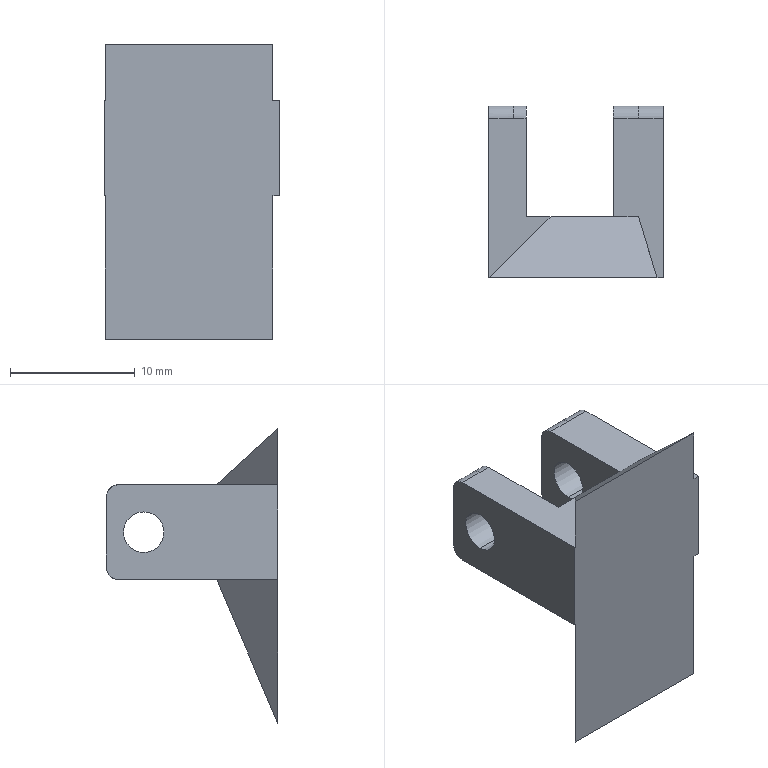Part | SolidWorks | features MirrorStock 1 | 1 solid | 30 faces | box 14 x 13.739 x 23.602 mm | volume 1371 mm3 | plane 18 | cylinder 10 | spline 2 | commonest cylinder face diameters 2 x6 3.25 x4
STEP:
#1=CARTESIAN_POINT('',(-8.5,5.85,-5.425));
#2=VERTEX_POINT('',#1);
#3=CARTESIAN_POINT('',(-8.5,5.85,-2.175));
#4=VERTEX_POINT('',#3);
#5=CARTESIAN_POINT('',(-8.5,5.85,-3.8));
#6=DIRECTION('',(1.,0.,0.));
#7=DIRECTION('',(0.,0.,-1.));
#8=AXIS2_PLACEMENT_3D('',#5,#6,#7);
#9=CIRCLE('',#8,1.625);
#10=EDGE_CURVE('',#2,#4,#9,.T.);
#11=ORIENTED_EDGE('',*,*,#10,.F.);
#12=CARTESIAN_POINT('',(-5.5,5.85,-5.425));
#13=VERTEX_POINT('',#12);
#14=CARTESIAN_POINT('',(-4.1,5.85,-5.425));
#15=DIRECTION('',(1.,0.,0.));
#16=VECTOR('',#15,1000.);
#17=LINE('',#14,#16);
#18=EDGE_CURVE('',#2,#13,#17,.T.);
#19=ORIENTED_EDGE('',*,*,#18,.T.);
#20=CARTESIAN_POINT('',(-5.5,5.85,-2.175));
#21=VERTEX_POINT('',#20);
#22=CARTESIAN_POINT('',(-5.5,5.85,-3.8));
#23=DIRECTION('',(-1.,0.,0.));
#24=DIRECTION('',(0.,0.,-1.));
#25=AXIS2_PLACEMENT_3D('',#22,#23,#24);
#26=CIRCLE('',#25,1.625);
#27=EDGE_CURVE('',#21,#13,#26,.T.);
#28=ORIENTED_EDGE('',*,*,#27,.F.);
#29=CARTESIAN_POINT('',(-4.1,5.85,-2.175));
#30=DIRECTION('',(1.,0.,0.));
#31=VECTOR('',#30,1000.);
#32=LINE('',#29,#31);
#33=EDGE_CURVE('',#4,#21,#32,.T.);
#34=ORIENTED_EDGE('',*,*,#33,.F.);
#35=EDGE_LOOP('',(#11,#19,#28,#34));
#36=FACE_OUTER_BOUND('',#35,.T.);
#37=CARTESIAN_POINT('',(-4.1,5.85,-3.8));
#38=DIRECTION('',(1.,0.,0.));
#39=DIRECTION('',(0.,0.,1.));
#40=AXIS2_PLACEMENT_3D('',#37,#38,#39);
#41=CYLINDRICAL_SURFACE('',#40,1.625);
#42=ADVANCED_FACE('',(#36),#41,.F.);
#43=CARTESIAN_POINT('',(1.5,5.85,-5.425));
#44=VERTEX_POINT('',#43);
#45=CARTESIAN_POINT('',(1.5,5.85,-2.175));
#46=VERTEX_POINT('',#45);
#47=CARTESIAN_POINT('',(1.5,5.85,-3.8));
#48=DIRECTION('',(1.,0.,0.));
#49=DIRECTION('',(0.,1.,0.));
#50=AXIS2_PLACEMENT_3D('',#47,#48,#49);
#51=CIRCLE('',#50,1.625);
#52=EDGE_CURVE('',#44,#46,#51,.T.);
#53=ORIENTED_EDGE('',*,*,#52,.F.);
#54=CARTESIAN_POINT('',(5.5,5.85,-5.425));
#55=VERTEX_POINT('',#54);
#56=CARTESIAN_POINT('',(-4.1,5.85,-5.425));
#57=DIRECTION('',(1.,0.,0.));
#58=VECTOR('',#57,1000.);
#59=LINE('',#56,#58);
#60=EDGE_CURVE('',#44,#55,#59,.T.);
#61=ORIENTED_EDGE('',*,*,#60,.T.);
#62=CARTESIAN_POINT('',(5.5,5.85,-2.175));
#63=VERTEX_POINT('',#62);
#64=CARTESIAN_POINT('',(5.5,5.85,-3.8));
#65=DIRECTION('',(-1.,0.,0.));
#66=DIRECTION('',(0.,0.,1.));
#67=AXIS2_PLACEMENT_3D('',#64,#65,#66);
#68=CIRCLE('',#67,1.625);
#69=EDGE_CURVE('',#63,#55,#68,.T.);
#70=ORIENTED_EDGE('',*,*,#69,.F.);
#71=CARTESIAN_POINT('',(-4.1,5.85,-2.175));
#72=DIRECTION('',(1.,0.,0.));
#73=VECTOR('',#72,1000.);
#74=LINE('',#71,#73);
#75=EDGE_CURVE('',#46,#63,#74,.T.);
#76=ORIENTED_EDGE('',*,*,#75,.F.);
#77=EDGE_LOOP('',(#53,#61,#70,#76));
#78=FACE_OUTER_BOUND('',#77,.T.);
#79=CARTESIAN_POINT('',(-4.1,5.85,-3.8));
#80=DIRECTION('',(1.,0.,0.));
#81=DIRECTION('',(0.,0.,1.));
#82=AXIS2_PLACEMENT_3D('',#79,#80,#81);
#83=CYLINDRICAL_SURFACE('',#82,1.625);
#84=ADVANCED_FACE('',(#78),#83,.F.);
#85=CARTESIAN_POINT('',(-3.5,0.,0.));
#86=VERTEX_POINT('',#85);
#87=CARTESIAN_POINT('',(-8.444,-4.889,4.494));
#88=VERTEX_POINT('',#87);
#89=CARTESIAN_POINT('',(-7.066,-3.527,3.241));
#90=DIRECTION('',(-0.5972,-0.5906,0.5428));
#91=VECTOR('',#90,1000.);
#92=LINE('',#89,#91);
#93=EDGE_CURVE('',#86,#88,#92,.T.);
#94=ORIENTED_EDGE('',*,*,#93,.F.);
#95=CARTESIAN_POINT('',(-8.444,-4.889,0.));
#96=VERTEX_POINT('',#95);
#97=CARTESIAN_POINT('',(-3.5,0.,0.));
#98=DIRECTION('',(-0.711,-0.7032,0.));
#99=VECTOR('',#98,1000.);
#100=LINE('',#97,#99);
#101=EDGE_CURVE('',#86,#96,#100,.T.);
#102=ORIENTED_EDGE('',*,*,#101,.T.);
#103=CARTESIAN_POINT('',(-8.444,-4.889,14.285));
#104=DIRECTION('',(0.,0.,-1.));
#105=VECTOR('',#104,1000.);
#106=LINE('',#103,#105);
#107=EDGE_CURVE('',#88,#96,#106,.T.);
#108=ORIENTED_EDGE('',*,*,#107,.F.);
#109=EDGE_LOOP('',(#94,#102,#108));
#110=FACE_OUTER_BOUND('',#109,.T.);
#111=CARTESIAN_POINT('',(-3.5,0.,14.285));
#112=DIRECTION('',(0.7032,-0.711,0.));
#113=DIRECTION('',(0.711,0.7032,0.));
#114=AXIS2_PLACEMENT_3D('',#111,#112,#113);
#115=PLANE('',#114);
#116=ADVANCED_FACE('',(#110),#115,.F.);
#117=CARTESIAN_POINT('',(3.5,0.,-7.6));
#118=VERTEX_POINT('',#117);
#119=CARTESIAN_POINT('',(4.983,-4.889,-19.108));
#120=VERTEX_POINT('',#119);
#121=CARTESIAN_POINT('',(3.264,0.7776,-5.77));
#122=DIRECTION('',(0.1178,-0.3883,-0.914));
#123=VECTOR('',#122,1000.);
#124=LINE('',#121,#123);
#125=EDGE_CURVE('',#118,#120,#124,.T.);
#126=ORIENTED_EDGE('',*,*,#125,.F.);
#127=CARTESIAN_POINT('',(4.983,-4.889,-7.6));
#128=VERTEX_POINT('',#127);
#129=CARTESIAN_POINT('',(3.5,0.,-7.6));
#130=DIRECTION('',(-0.2903,0.9569,0.));
#131=VECTOR('',#130,1000.);
#132=LINE('',#129,#131);
#133=EDGE_CURVE('',#128,#118,#132,.T.);
#134=ORIENTED_EDGE('',*,*,#133,.F.);
#135=CARTESIAN_POINT('',(4.983,-4.889,14.285));
#136=DIRECTION('',(0.,0.,1.));
#137=VECTOR('',#136,1000.);
#138=LINE('',#135,#137);
#139=EDGE_CURVE('',#120,#128,#138,.T.);
#140=ORIENTED_EDGE('',*,*,#139,.F.);
#141=EDGE_LOOP('',(#126,#134,#140));
#142=FACE_OUTER_BOUND('',#141,.T.);
#143=CARTESIAN_POINT('',(3.5,0.,14.285));
#144=DIRECTION('',(-0.9569,-0.2903,0.));
#145=DIRECTION('',(0.2903,-0.9569,0.));
#146=AXIS2_PLACEMENT_3D('',#143,#144,#145);
#147=PLANE('',#146);
#148=ADVANCED_FACE('',(#142),#147,.F.);
#149=ORIENTED_EDGE('',*,*,#133,.T.);
#150=CARTESIAN_POINT('',(1.5,0.,-7.6));
#151=VERTEX_POINT('',#150);
#152=CARTESIAN_POINT('',(0.,0.,-7.6));
#153=DIRECTION('',(1.,0.,0.));
#154=VECTOR('',#153,1000.);
#155=LINE('',#152,#154);
#156=EDGE_CURVE('',#151,#118,#155,.T.);
#157=ORIENTED_EDGE('',*,*,#156,.F.);
#158=CARTESIAN_POINT('',(1.5,7.85,-7.6));
#159=VERTEX_POINT('',#158);
#160=CARTESIAN_POINT('',(1.5,8.85,-7.6));
#161=DIRECTION('',(0.,-1.,0.));
#162=VECTOR('',#161,1000.);
#163=LINE('',#160,#162);
#164=EDGE_CURVE('',#159,#151,#163,.T.);
#165=ORIENTED_EDGE('',*,*,#164,.F.);
#166=CARTESIAN_POINT('',(3.5,7.85,-7.6));
#167=VERTEX_POINT('',#166);
#168=CARTESIAN_POINT('',(0.,7.85,-7.6));
#169=DIRECTION('',(-1.,0.,0.));
#170=VECTOR('',#169,1000.);
#171=LINE('',#168,#170);
#172=EDGE_CURVE('',#167,#159,#171,.T.);
#173=ORIENTED_EDGE('',*,*,#172,.F.);
#174=CARTESIAN_POINT('',(5.5,7.85,-7.6));
#175=VERTEX_POINT('',#174);
#176=CARTESIAN_POINT('',(5.5,7.85,-7.6));
#177=CARTESIAN_POINT('',(4.833,7.85,-7.6));
#178=CARTESIAN_POINT('',(4.167,7.85,-7.6));
#179=CARTESIAN_POINT('',(3.5,7.85,-7.6));
#180=B_SPLINE_CURVE_WITH_KNOTS('',3,(#176,#177,#178,#179),.UNSPECIFIED.,.F.,.F.,(4,4),(0.,1.),.UNSPECIFIED.);
#181=EDGE_CURVE('',#175,#167,#180,.T.);
#182=ORIENTED_EDGE('',*,*,#181,.F.);
#183=CARTESIAN_POINT('',(5.5,-4.889,-7.6));
#184=VERTEX_POINT('',#183);
#185=CARTESIAN_POINT('',(5.5,-9.889,-7.6));
#186=DIRECTION('',(0.,1.,0.));
#187=VECTOR('',#186,1000.);
#188=LINE('',#185,#187);
#189=EDGE_CURVE('',#184,#175,#188,.T.);
#190=ORIENTED_EDGE('',*,*,#189,.F.);
#191=CARTESIAN_POINT('',(0.,-4.889,-7.6));
#192=DIRECTION('',(1.,0.,0.));
#193=VECTOR('',#192,1000.);
#194=LINE('',#191,#193);
#195=EDGE_CURVE('',#128,#184,#194,.T.);
#196=ORIENTED_EDGE('',*,*,#195,.F.);
#197=EDGE_LOOP('',(#149,#157,#165,#173,#182,#190,#196));
#198=FACE_OUTER_BOUND('',#197,.T.);
#199=CARTESIAN_POINT('',(0.,0.,-7.6));
#200=DIRECTION('',(0.,0.,1.));
#201=DIRECTION('',(-1.,0.,0.));
#202=AXIS2_PLACEMENT_3D('',#199,#200,#201);
#203=PLANE('',#202);
#204=ADVANCED_FACE('',(#198),#203,.F.);
#205=CARTESIAN_POINT('',(4.983,-4.889,0.));
#206=VERTEX_POINT('',#205);
#207=CARTESIAN_POINT('',(5.5,-4.889,0.));
#208=VERTEX_POINT('',#207);
#209=CARTESIAN_POINT('',(0.,-4.889,0.));
#210=DIRECTION('',(1.,0.,0.));
#211=VECTOR('',#210,1000.);
#212=LINE('',#209,#211);
#213=EDGE_CURVE('',#206,#208,#212,.T.);
#214=ORIENTED_EDGE('',*,*,#213,.T.);
#215=CARTESIAN_POINT('',(5.5,7.85,0.));
#216=VERTEX_POINT('',#215);
#217=CARTESIAN_POINT('',(5.5,-9.889,0.));
#218=DIRECTION('',(0.,1.,0.));
#219=VECTOR('',#218,1000.);
#220=LINE('',#217,#219);
#221=EDGE_CURVE('',#208,#216,#220,.T.);
#222=ORIENTED_EDGE('',*,*,#221,.T.);
#223=CARTESIAN_POINT('',(3.5,7.85,0.));
#224=VERTEX_POINT('',#223);
#225=CARTESIAN_POINT('',(0.,7.85,0.));
#226=DIRECTION('',(1.,0.,0.));
#227=VECTOR('',#226,1000.);
#228=LINE('',#225,#227);
#229=EDGE_CURVE('',#224,#216,#228,.T.);
#230=ORIENTED_EDGE('',*,*,#229,.F.);
#231=CARTESIAN_POINT('',(1.5,7.85,0.));
#232=VERTEX_POINT('',#231);
#233=CARTESIAN_POINT('',(0.,7.85,0.));
#234=DIRECTION('',(1.,0.,0.));
#235=VECTOR('',#234,1000.);
#236=LINE('',#233,#235);
#237=EDGE_CURVE('',#232,#224,#236,.T.);
#238=ORIENTED_EDGE('',*,*,#237,.F.);
#239=CARTESIAN_POINT('',(1.5,0.,0.));
#240=VERTEX_POINT('',#239);
#241=CARTESIAN_POINT('',(1.5,8.85,0.));
#242=DIRECTION('',(0.,-1.,0.));
#243=VECTOR('',#242,1000.);
#244=LINE('',#241,#243);
#245=EDGE_CURVE('',#232,#240,#244,.T.);
#246=ORIENTED_EDGE('',*,*,#245,.T.);
#247=CARTESIAN_POINT('',(3.5,0.,0.));
#248=VERTEX_POINT('',#247);
#249=CARTESIAN_POINT('',(3.5,0.,0.));
#250=DIRECTION('',(-1.,0.,0.));
#251=VECTOR('',#250,1000.);
#252=LINE('',#249,#251);
#253=EDGE_CURVE('',#248,#240,#252,.T.);
#254=ORIENTED_EDGE('',*,*,#253,.F.);
#255=CARTESIAN_POINT('',(3.5,0.,0.));
#256=DIRECTION('',(0.2903,-0.9569,0.));
#257=VECTOR('',#256,1000.);
#258=LINE('',#255,#257);
#259=EDGE_CURVE('',#248,#206,#258,.T.);
#260=ORIENTED_EDGE('',*,*,#259,.T.);
#261=EDGE_LOOP('',(#214,#222,#230,#238,#246,#254,#260));
#262=FACE_OUTER_BOUND('',#261,.T.);
#263=CARTESIAN_POINT('',(0.,0.,0.));
#264=DIRECTION('',(0.,0.,1.));
#265=DIRECTION('',(-1.,0.,0.));
#266=AXIS2_PLACEMENT_3D('',#263,#264,#265);
#267=PLANE('',#266);
#268=ADVANCED_FACE('',(#262),#267,.T.);
#269=ORIENTED_EDGE('',*,*,#229,.T.);
#270=CARTESIAN_POINT('',(5.5,8.85,-1.));
#271=VERTEX_POINT('',#270);
#272=CARTESIAN_POINT('',(5.5,7.85,-1.));
#273=DIRECTION('',(-1.,0.,0.));
#274=DIRECTION('',(0.,0.,1.));
#275=AXIS2_PLACEMENT_3D('',#272,#273,#274);
#276=CIRCLE('',#275,1.);
#277=EDGE_CURVE('',#216,#271,#276,.T.);
#278=ORIENTED_EDGE('',*,*,#277,.T.);
#279=CARTESIAN_POINT('',(3.5,8.85,-1.));
#280=VERTEX_POINT('',#279);
#281=CARTESIAN_POINT('',(0.,8.85,-1.));
#282=DIRECTION('',(-1.,0.,0.));
#283=VECTOR('',#282,1000.);
#284=LINE('',#281,#283);
#285=EDGE_CURVE('',#271,#280,#284,.T.);
#286=ORIENTED_EDGE('',*,*,#285,.T.);
#287=CARTESIAN_POINT('',(3.5,7.85,-1.));
#288=DIRECTION('',(-1.,0.,0.));
#289=DIRECTION('',(0.,0.,-1.));
#290=AXIS2_PLACEMENT_3D('',#287,#288,#289);
#291=CIRCLE('',#290,1.);
#292=EDGE_CURVE('',#224,#280,#291,.T.);
#293=ORIENTED_EDGE('',*,*,#292,.F.);
#294=EDGE_LOOP('',(#269,#278,#286,#293));
#295=FACE_OUTER_BOUND('',#294,.T.);
#296=CARTESIAN_POINT('',(0.,7.85,-1.));
#297=DIRECTION('',(-1.,0.,0.));
#298=DIRECTION('',(0.,0.,-1.));
#299=AXIS2_PLACEMENT_3D('',#296,#297,#298);
#300=CYLINDRICAL_SURFACE('',#299,1.);
#301=ADVANCED_FACE('',(#295),#300,.T.);
#302=CARTESIAN_POINT('',(-8.5,7.85,0.));
#303=VERTEX_POINT('',#302);
#304=CARTESIAN_POINT('',(-6.5,7.85,0.));
#305=VERTEX_POINT('',#304);
#306=CARTESIAN_POINT('',(-8.5,7.85,0.));
#307=CARTESIAN_POINT('',(-7.833,7.85,0.));
#308=CARTESIAN_POINT('',(-7.167,7.85,0.));
#309=CARTESIAN_POINT('',(-6.5,7.85,0.));
#310=B_SPLINE_CURVE_WITH_KNOTS('',3,(#306,#307,#308,#309),.UNSPECIFIED.,.F.,.F.,(4,4),(0.,1.),.UNSPECIFIED.);
#311=EDGE_CURVE('',#303,#305,#310,.T.);
#312=ORIENTED_EDGE('',*,*,#311,.T.);
#313=CARTESIAN_POINT('',(-6.5,8.85,-1.));
#314=VERTEX_POINT('',#313);
#315=CARTESIAN_POINT('',(-6.5,8.85,-1.));
#316=CARTESIAN_POINT('',(-6.5,8.85,-0.7382));
#317=CARTESIAN_POINT('',(-6.5,8.742,-0.478));
#318=CARTESIAN_POINT('',(-6.5,8.372,-0.1078));
#319=CARTESIAN_POINT('',(-6.5,8.112,0.));
#320=CARTESIAN_POINT('',(-6.5,7.85,0.));
#321=B_SPLINE_CURVE_WITH_KNOTS('',3,(#315,#316,#317,#318,#319,#320),.UNSPECIFIED.,.F.,.F.,(4,2,4),(0.,0.5,1.),.UNSPECIFIED.);
#322=EDGE_CURVE('',#314,#305,#321,.T.);
#323=ORIENTED_EDGE('',*,*,#322,.F.);
#324=CARTESIAN_POINT('',(-8.5,8.85,-1.));
#325=VERTEX_POINT('',#324);
#326=CARTESIAN_POINT('',(-6.5,8.85,-1.));
#327=CARTESIAN_POINT('',(-7.167,8.85,-1.));
#328=CARTESIAN_POINT('',(-7.833,8.85,-1.));
#329=CARTESIAN_POINT('',(-8.5,8.85,-1.));
#330=B_SPLINE_CURVE_WITH_KNOTS('',3,(#326,#327,#328,#329),.UNSPECIFIED.,.F.,.F.,(4,4),(0.,1.),.UNSPECIFIED.);
#331=EDGE_CURVE('',#314,#325,#330,.T.);
#332=ORIENTED_EDGE('',*,*,#331,.T.);
#333=CARTESIAN_POINT('',(-8.5,8.85,-1.));
#334=CARTESIAN_POINT('',(-8.5,8.85,0.));
#335=CARTESIAN_POINT('',(-8.5,7.85,0.));
#336=(BOUNDED_CURVE()B_SPLINE_CURVE(2,(#333,#334,#335),.UNSPECIFIED.,.F.,.F.)B_SPLINE_CURVE_WITH_KNOTS((3,3),(0.,1.),.UNSPECIFIED.)CURVE()GEOMETRIC_REPRESENTATION_ITEM()RATIONAL_B_SPLINE_CURVE((1.,0.7071,1.))REPRESENTATION_ITEM(''));
#337=EDGE_CURVE('',#325,#303,#336,.T.);
#338=ORIENTED_EDGE('',*,*,#337,.T.);
#339=EDGE_LOOP('',(#312,#323,#332,#338));
#340=FACE_OUTER_BOUND('',#339,.T.);
#341=CARTESIAN_POINT('',(-6.3,8.85,-1.));
#342=CARTESIAN_POINT('',(-6.367,8.85,-1.));
#343=CARTESIAN_POINT('',(-6.433,8.85,-1.));
#344=CARTESIAN_POINT('',(-7.167,8.85,-1.));
#345=CARTESIAN_POINT('',(-7.833,8.85,-1.));
#346=CARTESIAN_POINT('',(-8.567,8.85,-1.));
#347=CARTESIAN_POINT('',(-8.633,8.85,-1.));
#348=CARTESIAN_POINT('',(-8.7,8.85,-1.));
#349=CARTESIAN_POINT('',(-6.3,8.85,0.));
#350=CARTESIAN_POINT('',(-6.367,8.85,0.));
#351=CARTESIAN_POINT('',(-6.433,8.85,0.));
#352=CARTESIAN_POINT('',(-7.167,8.85,0.));
#353=CARTESIAN_POINT('',(-7.833,8.85,0.));
#354=CARTESIAN_POINT('',(-8.567,8.85,0.));
#355=CARTESIAN_POINT('',(-8.633,8.85,0.));
#356=CARTESIAN_POINT('',(-8.7,8.85,0.));
#357=CARTESIAN_POINT('',(-6.3,7.85,0.));
#358=CARTESIAN_POINT('',(-6.367,7.85,0.));
#359=CARTESIAN_POINT('',(-6.433,7.85,0.));
#360=CARTESIAN_POINT('',(-7.167,7.85,0.));
#361=CARTESIAN_POINT('',(-7.833,7.85,0.));
#362=CARTESIAN_POINT('',(-8.567,7.85,0.));
#363=CARTESIAN_POINT('',(-8.633,7.85,0.));
#364=CARTESIAN_POINT('',(-8.7,7.85,0.));
#365=(BOUNDED_SURFACE()B_SPLINE_SURFACE(2,3,((#341,#342,#343,#344,#345,#346,#347,#348),(#349,#350,#351,#352,#353,#354,#355,#356),(#357,#358,#359,#360,#361,#362,#363,#364)),.UNSPECIFIED.,.F.,.F.,.F.)B_SPLINE_SURFACE_WITH_KNOTS((3,3),(4,2,2,4),(0.,1.),(-0.1,0.,1.,1.1),.UNSPECIFIED.)GEOMETRIC_REPRESENTATION_ITEM()RATIONAL_B_SPLINE_SURFACE(((1.,1.,1.,1.,1.,1.,1.,1.),(0.7071,0.7071,0.7071,0.7071,0.7071,0.7071,0.7071,0.7071),(1.,1.,1.,1.,1.,1.,1.,1.)))REPRESENTATION_ITEM('')SURFACE());
#366=ADVANCED_FACE('',(#340),#365,.F.);
#367=CARTESIAN_POINT('',(-6.5,7.85,-7.6));
#368=VERTEX_POINT('',#367);
#369=CARTESIAN_POINT('',(-8.5,7.85,-7.6));
#370=VERTEX_POINT('',#369);
#371=CARTESIAN_POINT('',(0.,7.85,-7.6));
#372=DIRECTION('',(-1.,0.,0.));
#373=VECTOR('',#372,1000.);
#374=LINE('',#371,#373);
#375=EDGE_CURVE('',#368,#370,#374,.T.);
#376=ORIENTED_EDGE('',*,*,#375,.T.);
#377=CARTESIAN_POINT('',(-8.5,8.85,-6.6));
#378=VERTEX_POINT('',#377);
#379=CARTESIAN_POINT('',(-8.5,7.85,-6.6));
#380=DIRECTION('',(1.,0.,0.));
#381=DIRECTION('',(0.,0.,-1.));
#382=AXIS2_PLACEMENT_3D('',#379,#380,#381);
#383=CIRCLE('',#382,1.);
#384=EDGE_CURVE('',#370,#378,#383,.T.);
#385=ORIENTED_EDGE('',*,*,#384,.T.);
#386=CARTESIAN_POINT('',(-6.5,8.85,-6.6));
#387=VERTEX_POINT('',#386);
#388=CARTESIAN_POINT('',(-3.5,8.85,-6.6));
#389=DIRECTION('',(1.,0.,0.));
#390=VECTOR('',#389,1000.);
#391=LINE('',#388,#390);
#392=EDGE_CURVE('',#378,#387,#391,.T.);
#393=ORIENTED_EDGE('',*,*,#392,.T.);
#394=CARTESIAN_POINT('',(-6.5,7.85,-6.6));
#395=DIRECTION('',(1.,0.,0.));
#396=DIRECTION('',(0.,-1.,0.));
#397=AXIS2_PLACEMENT_3D('',#394,#395,#396);
#398=CIRCLE('',#397,1.);
#399=EDGE_CURVE('',#368,#387,#398,.T.);
#400=ORIENTED_EDGE('',*,*,#399,.F.);
#401=EDGE_LOOP('',(#376,#385,#393,#400));
#402=FACE_OUTER_BOUND('',#401,.T.);
#403=CARTESIAN_POINT('',(0.,7.85,-6.6));
#404=DIRECTION('',(-1.,0.,0.));
#405=DIRECTION('',(0.,0.,-1.));
#406=AXIS2_PLACEMENT_3D('',#403,#404,#405);
#407=CYLINDRICAL_SURFACE('',#406,1.);
#408=ADVANCED_FACE('',(#402),#407,.T.);
#409=ORIENTED_EDGE('',*,*,#181,.T.);
#410=CARTESIAN_POINT('',(3.5,8.85,-6.6));
#411=VERTEX_POINT('',#410);
#412=CARTESIAN_POINT('',(3.5,8.85,-6.6));
#413=CARTESIAN_POINT('',(3.5,8.85,-6.862));
#414=CARTESIAN_POINT('',(3.5,8.742,-7.122));
#415=CARTESIAN_POINT('',(3.5,8.372,-7.492));
#416=CARTESIAN_POINT('',(3.5,8.112,-7.6));
#417=CARTESIAN_POINT('',(3.5,7.85,-7.6));
#418=B_SPLINE_CURVE_WITH_KNOTS('',3,(#412,#413,#414,#415,#416,#417),.UNSPECIFIED.,.F.,.F.,(4,2,4),(0.,0.5,1.),.UNSPECIFIED.);
#419=EDGE_CURVE('',#411,#167,#418,.T.);
#420=ORIENTED_EDGE('',*,*,#419,.F.);
#421=CARTESIAN_POINT('',(5.5,8.85,-6.6));
#422=VERTEX_POINT('',#421);
#423=CARTESIAN_POINT('',(3.5,8.85,-6.6));
#424=CARTESIAN_POINT('',(4.167,8.85,-6.6));
#425=CARTESIAN_POINT('',(4.833,8.85,-6.6));
#426=CARTESIAN_POINT('',(5.5,8.85,-6.6));
#427=B_SPLINE_CURVE_WITH_KNOTS('',3,(#423,#424,#425,#426),.UNSPECIFIED.,.F.,.F.,(4,4),(0.,1.),.UNSPECIFIED.);
#428=EDGE_CURVE('',#411,#422,#427,.T.);
#429=ORIENTED_EDGE('',*,*,#428,.T.);
#430=CARTESIAN_POINT('',(5.5,8.85,-6.6));
#431=CARTESIAN_POINT('',(5.5,8.85,-7.6));
#432=CARTESIAN_POINT('',(5.5,7.85,-7.6));
#433=(BOUNDED_CURVE()B_SPLINE_CURVE(2,(#430,#431,#432),.UNSPECIFIED.,.F.,.F.)B_SPLINE_CURVE_WITH_KNOTS((3,3),(0.,1.),.UNSPECIFIED.)CURVE()GEOMETRIC_REPRESENTATION_ITEM()RATIONAL_B_SPLINE_CURVE((1.,0.7071,1.))REPRESENTATION_ITEM(''));
#434=EDGE_CURVE('',#422,#175,#433,.T.);
#435=ORIENTED_EDGE('',*,*,#434,.T.);
#436=EDGE_LOOP('',(#409,#420,#429,#435));
#437=FACE_OUTER_BOUND('',#436,.T.);
#438=CARTESIAN_POINT('',(3.3,8.85,-6.6));
#439=CARTESIAN_POINT('',(3.367,8.85,-6.6));
#440=CARTESIAN_POINT('',(3.433,8.85,-6.6));
#441=CARTESIAN_POINT('',(4.167,8.85,-6.6));
#442=CARTESIAN_POINT('',(4.833,8.85,-6.6));
#443=CARTESIAN_POINT('',(5.567,8.85,-6.6));
#444=CARTESIAN_POINT('',(5.633,8.85,-6.6));
#445=CARTESIAN_POINT('',(5.7,8.85,-6.6));
#446=CARTESIAN_POINT('',(3.3,8.85,-7.6));
#447=CARTESIAN_POINT('',(3.367,8.85,-7.6));
#448=CARTESIAN_POINT('',(3.433,8.85,-7.6));
#449=CARTESIAN_POINT('',(4.167,8.85,-7.6));
#450=CARTESIAN_POINT('',(4.833,8.85,-7.6));
#451=CARTESIAN_POINT('',(5.567,8.85,-7.6));
#452=CARTESIAN_POINT('',(5.633,8.85,-7.6));
#453=CARTESIAN_POINT('',(5.7,8.85,-7.6));
#454=CARTESIAN_POINT('',(3.3,7.85,-7.6));
#455=CARTESIAN_POINT('',(3.367,7.85,-7.6));
#456=CARTESIAN_POINT('',(3.433,7.85,-7.6));
#457=CARTESIAN_POINT('',(4.167,7.85,-7.6));
#458=CARTESIAN_POINT('',(4.833,7.85,-7.6));
#459=CARTESIAN_POINT('',(5.567,7.85,-7.6));
#460=CARTESIAN_POINT('',(5.633,7.85,-7.6));
#461=CARTESIAN_POINT('',(5.7,7.85,-7.6));
#462=(BOUNDED_SURFACE()B_SPLINE_SURFACE(2,3,((#438,#439,#440,#441,#442,#443,#444,#445),(#446,#447,#448,#449,#450,#451,#452,#453),(#454,#455,#456,#457,#458,#459,#460,#461)),.UNSPECIFIED.,.F.,.F.,.F.)B_SPLINE_SURFACE_WITH_KNOTS((3,3),(4,2,2,4),(0.,1.),(-0.1,0.,1.,1.1),.UNSPECIFIED.)GEOMETRIC_REPRESENTATION_ITEM()RATIONAL_B_SPLINE_SURFACE(((1.,1.,1.,1.,1.,1.,1.,1.),(0.7071,0.7071,0.7071,0.7071,0.7071,0.7071,0.7071,0.7071),(1.,1.,1.,1.,1.,1.,1.,1.)))REPRESENTATION_ITEM('')SURFACE());
#463=ADVANCED_FACE('',(#437),#462,.F.);
#464=CARTESIAN_POINT('',(-5.5,7.85,0.));
#465=VERTEX_POINT('',#464);
#466=CARTESIAN_POINT('',(-5.5,8.85,-1.));
#467=VERTEX_POINT('',#466);
#468=CARTESIAN_POINT('',(-5.5,7.85,-1.));
#469=DIRECTION('',(-1.,0.,0.));
#470=DIRECTION('',(0.,0.,-1.));
#471=AXIS2_PLACEMENT_3D('',#468,#469,#470);
#472=CIRCLE('',#471,1.);
#473=EDGE_CURVE('',#465,#467,#472,.T.);
#474=ORIENTED_EDGE('',*,*,#473,.T.);
#475=CARTESIAN_POINT('',(0.,8.85,-1.));
#476=DIRECTION('',(-1.,0.,0.));
#477=VECTOR('',#476,1000.);
#478=LINE('',#475,#477);
#479=EDGE_CURVE('',#467,#314,#478,.T.);
#480=ORIENTED_EDGE('',*,*,#479,.T.);
#481=ORIENTED_EDGE('',*,*,#322,.T.);
#482=CARTESIAN_POINT('',(0.,7.85,0.));
#483=DIRECTION('',(1.,0.,0.));
#484=VECTOR('',#483,1000.);
#485=LINE('',#482,#484);
#486=EDGE_CURVE('',#305,#465,#485,.T.);
#487=ORIENTED_EDGE('',*,*,#486,.T.);
#488=EDGE_LOOP('',(#474,#480,#481,#487));
#489=FACE_OUTER_BOUND('',#488,.T.);
#490=CARTESIAN_POINT('',(0.,7.85,-1.));
#491=DIRECTION('',(-1.,0.,0.));
#492=DIRECTION('',(0.,0.,-1.));
#493=AXIS2_PLACEMENT_3D('',#490,#491,#492);
#494=CYLINDRICAL_SURFACE('',#493,1.);
#495=ADVANCED_FACE('',(#489),#494,.T.);
#496=CARTESIAN_POINT('',(-5.5,8.85,-6.6));
#497=VERTEX_POINT('',#496);
#498=CARTESIAN_POINT('',(-5.5,7.85,-7.6));
#499=VERTEX_POINT('',#498);
#500=CARTESIAN_POINT('',(-5.5,7.85,-6.6));
#501=DIRECTION('',(-1.,0.,0.));
#502=DIRECTION('',(0.,0.,-1.));
#503=AXIS2_PLACEMENT_3D('',#500,#501,#502);
#504=CIRCLE('',#503,1.);
#505=EDGE_CURVE('',#497,#499,#504,.T.);
#506=ORIENTED_EDGE('',*,*,#505,.T.);
#507=CARTESIAN_POINT('',(0.,7.85,-7.6));
#508=DIRECTION('',(-1.,0.,0.));
#509=VECTOR('',#508,1000.);
#510=LINE('',#507,#509);
#511=EDGE_CURVE('',#499,#368,#510,.T.);
#512=ORIENTED_EDGE('',*,*,#511,.T.);
#513=ORIENTED_EDGE('',*,*,#399,.T.);
#514=CARTESIAN_POINT('',(-3.5,8.85,-6.6));
#515=DIRECTION('',(1.,0.,0.));
#516=VECTOR('',#515,1000.);
#517=LINE('',#514,#516);
#518=EDGE_CURVE('',#387,#497,#517,.T.);
#519=ORIENTED_EDGE('',*,*,#518,.T.);
#520=EDGE_LOOP('',(#506,#512,#513,#519));
#521=FACE_OUTER_BOUND('',#520,.T.);
#522=CARTESIAN_POINT('',(0.,7.85,-6.6));
#523=DIRECTION('',(-1.,0.,0.));
#524=DIRECTION('',(0.,0.,-1.));
#525=AXIS2_PLACEMENT_3D('',#522,#523,#524);
#526=CYLINDRICAL_SURFACE('',#525,1.);
#527=ADVANCED_FACE('',(#521),#526,.T.);
#528=CARTESIAN_POINT('',(-8.444,-4.889,-7.6));
#529=VERTEX_POINT('',#528);
#530=CARTESIAN_POINT('',(-3.5,0.,-7.6));
#531=VERTEX_POINT('',#530);
#532=CARTESIAN_POINT('',(-3.5,0.,-7.6));
#533=DIRECTION('',(0.711,0.7032,0.));
#534=VECTOR('',#533,1000.);
#535=LINE('',#532,#534);
#536=EDGE_CURVE('',#529,#531,#535,.T.);
#537=ORIENTED_EDGE('',*,*,#536,.T.);
#538=CARTESIAN_POINT('',(-8.444,-4.889,-19.108));
#539=VERTEX_POINT('',#538);
#540=CARTESIAN_POINT('',(-4.852,-1.337,-10.747));
#541=DIRECTION('',(0.3677,0.3636,0.8559));
#542=VECTOR('',#541,1000.);
#543=LINE('',#540,#542);
#544=EDGE_CURVE('',#539,#531,#543,.T.);
#545=ORIENTED_EDGE('',*,*,#544,.F.);
#546=CARTESIAN_POINT('',(-8.444,-4.889,14.285));
#547=DIRECTION('',(0.,0.,-1.));
#548=VECTOR('',#547,1000.);
#549=LINE('',#546,#548);
#550=EDGE_CURVE('',#529,#539,#549,.T.);
#551=ORIENTED_EDGE('',*,*,#550,.F.);
#552=EDGE_LOOP('',(#537,#545,#551));
#553=FACE_OUTER_BOUND('',#552,.T.);
#554=CARTESIAN_POINT('',(-3.5,0.,14.285));
#555=DIRECTION('',(0.7032,-0.711,0.));
#556=DIRECTION('',(0.711,0.7032,0.));
#557=AXIS2_PLACEMENT_3D('',#554,#555,#556);
#558=PLANE('',#557);
#559=ADVANCED_FACE('',(#553),#558,.F.);
#560=ORIENTED_EDGE('',*,*,#172,.T.);
#561=CARTESIAN_POINT('',(1.5,8.85,-6.6));
#562=VERTEX_POINT('',#561);
#563=CARTESIAN_POINT('',(1.5,7.85,-6.6));
#564=DIRECTION('',(1.,0.,0.));
#565=DIRECTION('',(0.,1.,0.));
#566=AXIS2_PLACEMENT_3D('',#563,#564,#565);
#567=CIRCLE('',#566,1.);
#568=EDGE_CURVE('',#159,#562,#567,.T.);
#569=ORIENTED_EDGE('',*,*,#568,.T.);
#570=CARTESIAN_POINT('',(-3.5,8.85,-6.6));
#571=DIRECTION('',(1.,0.,0.));
#572=VECTOR('',#571,1000.);
#573=LINE('',#570,#572);
#574=EDGE_CURVE('',#562,#411,#573,.T.);
#575=ORIENTED_EDGE('',*,*,#574,.T.);
#576=ORIENTED_EDGE('',*,*,#419,.T.);
#577=EDGE_LOOP('',(#560,#569,#575,#576));
#578=FACE_OUTER_BOUND('',#577,.T.);
#579=CARTESIAN_POINT('',(0.,7.85,-6.6));
#580=DIRECTION('',(-1.,0.,0.));
#581=DIRECTION('',(0.,0.,-1.));
#582=AXIS2_PLACEMENT_3D('',#579,#580,#581);
#583=CYLINDRICAL_SURFACE('',#582,1.);
#584=ADVANCED_FACE('',(#578),#583,.T.);
#585=ORIENTED_EDGE('',*,*,#237,.T.);
#586=ORIENTED_EDGE('',*,*,#292,.T.);
#587=CARTESIAN_POINT('',(1.5,8.85,-1.));
#588=VERTEX_POINT('',#587);
#589=CARTESIAN_POINT('',(0.,8.85,-1.));
#590=DIRECTION('',(-1.,0.,0.));
#591=VECTOR('',#590,1000.);
#592=LINE('',#589,#591);
#593=EDGE_CURVE('',#280,#588,#592,.T.);
#594=ORIENTED_EDGE('',*,*,#593,.T.);
#595=CARTESIAN_POINT('',(1.5,7.85,-1.));
#596=DIRECTION('',(1.,0.,0.));
#597=DIRECTION('',(0.,1.,0.));
#598=AXIS2_PLACEMENT_3D('',#595,#596,#597);
#599=CIRCLE('',#598,1.);
#600=EDGE_CURVE('',#588,#232,#599,.T.);
#601=ORIENTED_EDGE('',*,*,#600,.T.);
#602=EDGE_LOOP('',(#585,#586,#594,#601));
#603=FACE_OUTER_BOUND('',#602,.T.);
#604=CARTESIAN_POINT('',(0.,7.85,-1.));
#605=DIRECTION('',(-1.,0.,0.));
#606=DIRECTION('',(0.,0.,-1.));
#607=AXIS2_PLACEMENT_3D('',#604,#605,#606);
#608=CYLINDRICAL_SURFACE('',#607,1.);
#609=ADVANCED_FACE('',(#603),#608,.T.);
#610=CARTESIAN_POINT('',(5.5,8.85,0.));
#611=DIRECTION('',(0.,0.,1.));
#612=VECTOR('',#611,1000.);
#613=LINE('',#610,#612);
#614=EDGE_CURVE('',#422,#271,#613,.T.);
#615=ORIENTED_EDGE('',*,*,#614,.F.);
#616=ORIENTED_EDGE('',*,*,#428,.F.);
#617=ORIENTED_EDGE('',*,*,#574,.F.);
#618=CARTESIAN_POINT('',(1.5,8.85,-7.6));
#619=DIRECTION('',(0.,0.,1.));
#620=VECTOR('',#619,1000.);
#621=LINE('',#618,#620);
#622=EDGE_CURVE('',#562,#588,#621,.T.);
#623=ORIENTED_EDGE('',*,*,#622,.T.);
#624=ORIENTED_EDGE('',*,*,#593,.F.);
#625=ORIENTED_EDGE('',*,*,#285,.F.);
#626=EDGE_LOOP('',(#615,#616,#617,#623,#624,#625));
#627=FACE_OUTER_BOUND('',#626,.T.);
#628=CARTESIAN_POINT('',(-3.5,8.85,-7.6));
#629=DIRECTION('',(0.,-1.,0.));
#630=DIRECTION('',(0.,0.,1.));
#631=AXIS2_PLACEMENT_3D('',#628,#629,#630);
#632=PLANE('',#631);
#633=ADVANCED_FACE('',(#627),#632,.F.);
#634=ORIENTED_EDGE('',*,*,#60,.F.);
#635=CARTESIAN_POINT('',(1.5,5.85,-3.8));
#636=DIRECTION('',(1.,0.,0.));
#637=DIRECTION('',(0.,1.,0.));
#638=AXIS2_PLACEMENT_3D('',#635,#636,#637);
#639=CIRCLE('',#638,1.625);
#640=EDGE_CURVE('',#46,#44,#639,.T.);
#641=ORIENTED_EDGE('',*,*,#640,.F.);
#642=ORIENTED_EDGE('',*,*,#75,.T.);
#643=CARTESIAN_POINT('',(5.5,5.85,-3.8));
#644=DIRECTION('',(-1.,0.,0.));
#645=DIRECTION('',(0.,0.,1.));
#646=AXIS2_PLACEMENT_3D('',#643,#644,#645);
#647=CIRCLE('',#646,1.625);
#648=EDGE_CURVE('',#55,#63,#647,.T.);
#649=ORIENTED_EDGE('',*,*,#648,.F.);
#650=EDGE_LOOP('',(#634,#641,#642,#649));
#651=FACE_OUTER_BOUND('',#650,.T.);
#652=CARTESIAN_POINT('',(-4.1,5.85,-3.8));
#653=DIRECTION('',(1.,0.,0.));
#654=DIRECTION('',(0.,0.,1.));
#655=AXIS2_PLACEMENT_3D('',#652,#653,#654);
#656=CYLINDRICAL_SURFACE('',#655,1.625);
#657=ADVANCED_FACE('',(#651),#656,.F.);
#658=ORIENTED_EDGE('',*,*,#518,.F.);
#659=ORIENTED_EDGE('',*,*,#392,.F.);
#660=CARTESIAN_POINT('',(-8.5,8.85,0.));
#661=DIRECTION('',(0.,0.,-1.));
#662=VECTOR('',#661,1000.);
#663=LINE('',#660,#662);
#664=EDGE_CURVE('',#325,#378,#663,.T.);
#665=ORIENTED_EDGE('',*,*,#664,.F.);
#666=ORIENTED_EDGE('',*,*,#331,.F.);
#667=ORIENTED_EDGE('',*,*,#479,.F.);
#668=CARTESIAN_POINT('',(-5.5,8.85,-30.877));
#669=DIRECTION('',(0.,0.,1.));
#670=VECTOR('',#669,1000.);
#671=LINE('',#668,#670);
#672=EDGE_CURVE('',#497,#467,#671,.T.);
#673=ORIENTED_EDGE('',*,*,#672,.F.);
#674=EDGE_LOOP('',(#658,#659,#665,#666,#667,#673));
#675=FACE_OUTER_BOUND('',#674,.T.);
#676=CARTESIAN_POINT('',(-3.5,8.85,-7.6));
#677=DIRECTION('',(0.,-1.,0.));
#678=DIRECTION('',(0.,0.,1.));
#679=AXIS2_PLACEMENT_3D('',#676,#677,#678);
#680=PLANE('',#679);
#681=ADVANCED_FACE('',(#675),#680,.F.);
#682=CARTESIAN_POINT('',(-8.5,-4.889,-7.6));
#683=VERTEX_POINT('',#682);
#684=CARTESIAN_POINT('',(-8.5,-9.889,-7.6));
#685=DIRECTION('',(0.,1.,0.));
#686=VECTOR('',#685,1000.);
#687=LINE('',#684,#686);
#688=EDGE_CURVE('',#683,#370,#687,.T.);
#689=ORIENTED_EDGE('',*,*,#688,.T.);
#690=ORIENTED_EDGE('',*,*,#375,.F.);
#691=ORIENTED_EDGE('',*,*,#511,.F.);
#692=CARTESIAN_POINT('',(-5.5,0.,-7.6));
#693=VERTEX_POINT('',#692);
#694=CARTESIAN_POINT('',(-5.5,0.,-7.6));
#695=DIRECTION('',(0.,1.,0.));
#696=VECTOR('',#695,1000.);
#697=LINE('',#694,#696);
#698=EDGE_CURVE('',#693,#499,#697,.T.);
#699=ORIENTED_EDGE('',*,*,#698,.F.);
#700=CARTESIAN_POINT('',(0.,0.,-7.6));
#701=DIRECTION('',(-1.,0.,0.));
#702=VECTOR('',#701,1000.);
#703=LINE('',#700,#702);
#704=EDGE_CURVE('',#531,#693,#703,.T.);
#705=ORIENTED_EDGE('',*,*,#704,.F.);
#706=ORIENTED_EDGE('',*,*,#536,.F.);
#707=CARTESIAN_POINT('',(0.,-4.889,-7.6));
#708=DIRECTION('',(1.,0.,0.));
#709=VECTOR('',#708,1000.);
#710=LINE('',#707,#709);
#711=EDGE_CURVE('',#683,#529,#710,.T.);
#712=ORIENTED_EDGE('',*,*,#711,.F.);
#713=EDGE_LOOP('',(#689,#690,#691,#699,#705,#706,#712));
#714=FACE_OUTER_BOUND('',#713,.T.);
#715=CARTESIAN_POINT('',(0.,0.,-7.6));
#716=DIRECTION('',(0.,0.,1.));
#717=DIRECTION('',(-1.,0.,0.));
#718=AXIS2_PLACEMENT_3D('',#715,#716,#717);
#719=PLANE('',#718);
#720=ADVANCED_FACE('',(#714),#719,.F.);
#721=CARTESIAN_POINT('',(-8.5,-4.889,0.));
#722=VERTEX_POINT('',#721);
#723=CARTESIAN_POINT('',(0.,-4.889,0.));
#724=DIRECTION('',(1.,0.,0.));
#725=VECTOR('',#724,1000.);
#726=LINE('',#723,#725);
#727=EDGE_CURVE('',#722,#96,#726,.T.);
#728=ORIENTED_EDGE('',*,*,#727,.T.);
#729=ORIENTED_EDGE('',*,*,#101,.F.);
#730=CARTESIAN_POINT('',(-5.5,0.,0.));
#731=VERTEX_POINT('',#730);
#732=CARTESIAN_POINT('',(1.5,0.,0.));
#733=DIRECTION('',(-1.,0.,0.));
#734=VECTOR('',#733,1000.);
#735=LINE('',#732,#734);
#736=EDGE_CURVE('',#86,#731,#735,.T.);
#737=ORIENTED_EDGE('',*,*,#736,.T.);
#738=CARTESIAN_POINT('',(-5.5,1.85,0.));
#739=DIRECTION('',(0.,1.,0.));
#740=VECTOR('',#739,1000.);
#741=LINE('',#738,#740);
#742=EDGE_CURVE('',#731,#465,#741,.T.);
#743=ORIENTED_EDGE('',*,*,#742,.T.);
#744=ORIENTED_EDGE('',*,*,#486,.F.);
#745=ORIENTED_EDGE('',*,*,#311,.F.);
#746=CARTESIAN_POINT('',(-8.5,-9.889,0.));
#747=DIRECTION('',(0.,1.,0.));
#748=VECTOR('',#747,1000.);
#749=LINE('',#746,#748);
#750=EDGE_CURVE('',#722,#303,#749,.T.);
#751=ORIENTED_EDGE('',*,*,#750,.F.);
#752=EDGE_LOOP('',(#728,#729,#737,#743,#744,#745,#751));
#753=FACE_OUTER_BOUND('',#752,.T.);
#754=CARTESIAN_POINT('',(0.,0.,0.));
#755=DIRECTION('',(0.,0.,1.));
#756=DIRECTION('',(-1.,0.,0.));
#757=AXIS2_PLACEMENT_3D('',#754,#755,#756);
#758=PLANE('',#757);
#759=ADVANCED_FACE('',(#753),#758,.T.);
#760=ORIENTED_EDGE('',*,*,#18,.F.);
#761=CARTESIAN_POINT('',(-8.5,5.85,-3.8));
#762=DIRECTION('',(1.,0.,0.));
#763=DIRECTION('',(0.,0.,-1.));
#764=AXIS2_PLACEMENT_3D('',#761,#762,#763);
#765=CIRCLE('',#764,1.625);
#766=EDGE_CURVE('',#4,#2,#765,.T.);
#767=ORIENTED_EDGE('',*,*,#766,.F.);
#768=ORIENTED_EDGE('',*,*,#33,.T.);
#769=CARTESIAN_POINT('',(-5.5,5.85,-3.8));
#770=DIRECTION('',(-1.,0.,0.));
#771=DIRECTION('',(0.,0.,-1.));
#772=AXIS2_PLACEMENT_3D('',#769,#770,#771);
#773=CIRCLE('',#772,1.625);
#774=EDGE_CURVE('',#13,#21,#773,.T.);
#775=ORIENTED_EDGE('',*,*,#774,.F.);
#776=EDGE_LOOP('',(#760,#767,#768,#775));
#777=FACE_OUTER_BOUND('',#776,.T.);
#778=CARTESIAN_POINT('',(-4.1,5.85,-3.8));
#779=DIRECTION('',(1.,0.,0.));
#780=DIRECTION('',(0.,0.,1.));
#781=AXIS2_PLACEMENT_3D('',#778,#779,#780);
#782=CYLINDRICAL_SURFACE('',#781,1.625);
#783=ADVANCED_FACE('',(#777),#782,.F.);
#784=ORIENTED_EDGE('',*,*,#164,.T.);
#785=CARTESIAN_POINT('',(1.5,0.,-10.));
#786=DIRECTION('',(0.,0.,1.));
#787=VECTOR('',#786,1000.);
#788=LINE('',#785,#787);
#789=EDGE_CURVE('',#151,#240,#788,.T.);
#790=ORIENTED_EDGE('',*,*,#789,.T.);
#791=ORIENTED_EDGE('',*,*,#245,.F.);
#792=ORIENTED_EDGE('',*,*,#600,.F.);
#793=ORIENTED_EDGE('',*,*,#622,.F.);
#794=ORIENTED_EDGE('',*,*,#568,.F.);
#795=EDGE_LOOP('',(#784,#790,#791,#792,#793,#794));
#796=FACE_OUTER_BOUND('',#795,.T.);
#797=ORIENTED_EDGE('',*,*,#640,.T.);
#798=ORIENTED_EDGE('',*,*,#52,.T.);
#799=EDGE_LOOP('',(#797,#798));
#800=FACE_BOUND('',#799,.T.);
#801=CARTESIAN_POINT('',(1.5,8.85,-7.6));
#802=DIRECTION('',(1.,0.,0.));
#803=DIRECTION('',(0.,1.,0.));
#804=AXIS2_PLACEMENT_3D('',#801,#802,#803);
#805=PLANE('',#804);
#806=ADVANCED_FACE('',(#796,#800),#805,.F.);
#807=CARTESIAN_POINT('',(4.983,-4.889,4.494));
#808=VERTEX_POINT('',#807);
#809=CARTESIAN_POINT('',(-13.5,-4.889,4.494));
#810=DIRECTION('',(1.,0.,0.));
#811=VECTOR('',#810,1000.);
#812=LINE('',#809,#811);
#813=EDGE_CURVE('',#88,#808,#812,.T.);
#814=ORIENTED_EDGE('',*,*,#813,.T.);
#815=CARTESIAN_POINT('',(2.692,2.663,-2.447));
#816=DIRECTION('',(-0.218,0.7186,-0.6604));
#817=VECTOR('',#816,1000.);
#818=LINE('',#815,#817);
#819=EDGE_CURVE('',#808,#248,#818,.T.);
#820=ORIENTED_EDGE('',*,*,#819,.T.);
#821=ORIENTED_EDGE('',*,*,#253,.T.);
#822=CARTESIAN_POINT('',(1.5,0.,0.));
#823=DIRECTION('',(-1.,0.,0.));
#824=VECTOR('',#823,1000.);
#825=LINE('',#822,#824);
#826=EDGE_CURVE('',#240,#86,#825,.T.);
#827=ORIENTED_EDGE('',*,*,#826,.T.);
#828=ORIENTED_EDGE('',*,*,#93,.T.);
#829=EDGE_LOOP('',(#814,#820,#821,#827,#828));
#830=FACE_OUTER_BOUND('',#829,.T.);
#831=CARTESIAN_POINT('',(-13.5,0.,0.));
#832=DIRECTION('',(0.,0.6767,0.7363));
#833=DIRECTION('',(0.,0.7363,-0.6767));
#834=AXIS2_PLACEMENT_3D('',#831,#832,#833);
#835=PLANE('',#834);
#836=ADVANCED_FACE('',(#830),#835,.T.);
#837=CARTESIAN_POINT('',(-13.5,-4.889,-19.108));
#838=DIRECTION('',(-1.,0.,0.));
#839=VECTOR('',#838,1000.);
#840=LINE('',#837,#839);
#841=EDGE_CURVE('',#120,#539,#840,.T.);
#842=ORIENTED_EDGE('',*,*,#841,.T.);
#843=ORIENTED_EDGE('',*,*,#544,.T.);
#844=CARTESIAN_POINT('',(0.,0.,-7.6));
#845=DIRECTION('',(1.,0.,0.));
#846=VECTOR('',#845,1000.);
#847=LINE('',#844,#846);
#848=EDGE_CURVE('',#531,#151,#847,.T.);
#849=ORIENTED_EDGE('',*,*,#848,.T.);
#850=ORIENTED_EDGE('',*,*,#156,.T.);
#851=ORIENTED_EDGE('',*,*,#125,.T.);
#852=EDGE_LOOP('',(#842,#843,#849,#850,#851));
#853=FACE_OUTER_BOUND('',#852,.T.);
#854=CARTESIAN_POINT('',(-13.5,0.,-7.6));
#855=DIRECTION('',(0.,0.9204,-0.391));
#856=DIRECTION('',(0.,-0.391,-0.9204));
#857=AXIS2_PLACEMENT_3D('',#854,#855,#856);
#858=PLANE('',#857);
#859=ADVANCED_FACE('',(#853),#858,.T.);
#860=ORIENTED_EDGE('',*,*,#259,.F.);
#861=ORIENTED_EDGE('',*,*,#819,.F.);
#862=CARTESIAN_POINT('',(4.983,-4.889,14.285));
#863=DIRECTION('',(0.,0.,1.));
#864=VECTOR('',#863,1000.);
#865=LINE('',#862,#864);
#866=EDGE_CURVE('',#206,#808,#865,.T.);
#867=ORIENTED_EDGE('',*,*,#866,.F.);
#868=EDGE_LOOP('',(#860,#861,#867));
#869=FACE_OUTER_BOUND('',#868,.T.);
#870=CARTESIAN_POINT('',(3.5,0.,14.285));
#871=DIRECTION('',(-0.9569,-0.2903,0.));
#872=DIRECTION('',(0.2903,-0.9569,0.));
#873=AXIS2_PLACEMENT_3D('',#870,#871,#872);
#874=PLANE('',#873);
#875=ADVANCED_FACE('',(#869),#874,.F.);
#876=CARTESIAN_POINT('',(-8.5,-4.889,0.));
#877=DIRECTION('',(0.,0.,1.));
#878=VECTOR('',#877,1000.);
#879=LINE('',#876,#878);
#880=EDGE_CURVE('',#683,#722,#879,.T.);
#881=ORIENTED_EDGE('',*,*,#880,.T.);
#882=ORIENTED_EDGE('',*,*,#750,.T.);
#883=ORIENTED_EDGE('',*,*,#337,.F.);
#884=ORIENTED_EDGE('',*,*,#664,.T.);
#885=ORIENTED_EDGE('',*,*,#384,.F.);
#886=ORIENTED_EDGE('',*,*,#688,.F.);
#887=EDGE_LOOP('',(#881,#882,#883,#884,#885,#886));
#888=FACE_OUTER_BOUND('',#887,.T.);
#889=ORIENTED_EDGE('',*,*,#766,.T.);
#890=ORIENTED_EDGE('',*,*,#10,.T.);
#891=EDGE_LOOP('',(#889,#890));
#892=FACE_BOUND('',#891,.T.);
#893=CARTESIAN_POINT('',(-8.5,-9.889,0.));
#894=DIRECTION('',(-1.,0.,0.));
#895=DIRECTION('',(0.,0.,-1.));
#896=AXIS2_PLACEMENT_3D('',#893,#894,#895);
#897=PLANE('',#896);
#898=ADVANCED_FACE('',(#888,#892),#897,.T.);
#899=CARTESIAN_POINT('',(5.5,-4.889,0.));
#900=DIRECTION('',(0.,0.,-1.));
#901=VECTOR('',#900,1000.);
#902=LINE('',#899,#901);
#903=EDGE_CURVE('',#208,#184,#902,.T.);
#904=ORIENTED_EDGE('',*,*,#903,.T.);
#905=ORIENTED_EDGE('',*,*,#189,.T.);
#906=ORIENTED_EDGE('',*,*,#434,.F.);
#907=ORIENTED_EDGE('',*,*,#614,.T.);
#908=ORIENTED_EDGE('',*,*,#277,.F.);
#909=ORIENTED_EDGE('',*,*,#221,.F.);
#910=EDGE_LOOP('',(#904,#905,#906,#907,#908,#909));
#911=FACE_OUTER_BOUND('',#910,.T.);
#912=ORIENTED_EDGE('',*,*,#69,.T.);
#913=ORIENTED_EDGE('',*,*,#648,.T.);
#914=EDGE_LOOP('',(#912,#913));
#915=FACE_BOUND('',#914,.T.);
#916=CARTESIAN_POINT('',(5.5,-9.889,0.));
#917=DIRECTION('',(1.,0.,0.));
#918=DIRECTION('',(0.,0.,1.));
#919=AXIS2_PLACEMENT_3D('',#916,#917,#918);
#920=PLANE('',#919);
#921=ADVANCED_FACE('',(#911,#915),#920,.T.);
#922=ORIENTED_EDGE('',*,*,#473,.F.);
#923=ORIENTED_EDGE('',*,*,#742,.F.);
#924=CARTESIAN_POINT('',(-5.5,0.,-10.));
#925=DIRECTION('',(0.,0.,1.));
#926=VECTOR('',#925,1000.);
#927=LINE('',#924,#926);
#928=EDGE_CURVE('',#693,#731,#927,.T.);
#929=ORIENTED_EDGE('',*,*,#928,.F.);
#930=ORIENTED_EDGE('',*,*,#698,.T.);
#931=ORIENTED_EDGE('',*,*,#505,.F.);
#932=ORIENTED_EDGE('',*,*,#672,.T.);
#933=EDGE_LOOP('',(#922,#923,#929,#930,#931,#932));
#934=FACE_OUTER_BOUND('',#933,.T.);
#935=ORIENTED_EDGE('',*,*,#27,.T.);
#936=ORIENTED_EDGE('',*,*,#774,.T.);
#937=EDGE_LOOP('',(#935,#936));
#938=FACE_BOUND('',#937,.T.);
#939=CARTESIAN_POINT('',(-5.5,1.85,-30.877));
#940=DIRECTION('',(-1.,0.,0.));
#941=DIRECTION('',(0.,0.,-1.));
#942=AXIS2_PLACEMENT_3D('',#939,#940,#941);
#943=PLANE('',#942);
#944=ADVANCED_FACE('',(#934,#938),#943,.F.);
#945=ORIENTED_EDGE('',*,*,#848,.F.);
#946=ORIENTED_EDGE('',*,*,#704,.T.);
#947=ORIENTED_EDGE('',*,*,#928,.T.);
#948=ORIENTED_EDGE('',*,*,#736,.F.);
#949=ORIENTED_EDGE('',*,*,#826,.F.);
#950=ORIENTED_EDGE('',*,*,#789,.F.);
#951=EDGE_LOOP('',(#945,#946,#947,#948,#949,#950));
#952=FACE_OUTER_BOUND('',#951,.T.);
#953=CARTESIAN_POINT('',(1.5,0.,-10.));
#954=DIRECTION('',(0.,-1.,0.));
#955=DIRECTION('',(0.,0.,1.));
#956=AXIS2_PLACEMENT_3D('',#953,#954,#955);
#957=PLANE('',#956);
#958=ADVANCED_FACE('',(#952),#957,.F.);
#959=ORIENTED_EDGE('',*,*,#880,.F.);
#960=ORIENTED_EDGE('',*,*,#711,.T.);
#961=ORIENTED_EDGE('',*,*,#550,.T.);
#962=ORIENTED_EDGE('',*,*,#841,.F.);
#963=ORIENTED_EDGE('',*,*,#139,.T.);
#964=ORIENTED_EDGE('',*,*,#195,.T.);
#965=ORIENTED_EDGE('',*,*,#903,.F.);
#966=ORIENTED_EDGE('',*,*,#213,.F.);
#967=ORIENTED_EDGE('',*,*,#866,.T.);
#968=ORIENTED_EDGE('',*,*,#813,.F.);
#969=ORIENTED_EDGE('',*,*,#107,.T.);
#970=ORIENTED_EDGE('',*,*,#727,.F.);
#971=EDGE_LOOP('',(#959,#960,#961,#962,#963,#964,#965,#966,#967,#968,#969,#970));
#972=FACE_OUTER_BOUND('',#971,.T.);
#973=CARTESIAN_POINT('',(-13.5,-4.889,6.783));
#974=DIRECTION('',(0.,1.,0.));
#975=DIRECTION('',(0.,0.,-1.));
#976=AXIS2_PLACEMENT_3D('',#973,#974,#975);
#977=PLANE('',#976);
#978=ADVANCED_FACE('',(#972),#977,.F.);
#979=CLOSED_SHELL('',(#42,#84,#116,#148,#204,#268,#301,#366,#408,#463,#495,#527,#559,#584,#609,#633,#657,#681,#720,#759,#783,#806,#836,#859,#875,#898,#921,#944,#958,#978));
#980=MANIFOLD_SOLID_BREP('',#979);
#981=CARTESIAN_POINT('',(0.,0.,0.));
#982=DIRECTION('',(0.,0.,1.));
#983=DIRECTION('',(1.,0.,0.));
#984=AXIS2_PLACEMENT_3D('',#981,#982,#983);
#985=(LENGTH_UNIT()NAMED_UNIT(*)SI_UNIT(.MILLI.,.METRE.));
#986=UNCERTAINTY_MEASURE_WITH_UNIT(LENGTH_MEASURE(0.00001),#985,'','');
#987=(NAMED_UNIT(*)PLANE_ANGLE_UNIT()SI_UNIT($,.RADIAN.));
#988=(NAMED_UNIT(*)SI_UNIT($,.STERADIAN.)SOLID_ANGLE_UNIT());
#989=(GEOMETRIC_REPRESENTATION_CONTEXT(3)GLOBAL_UNCERTAINTY_ASSIGNED_CONTEXT((#986))GLOBAL_UNIT_ASSIGNED_CONTEXT((#985,#987,#988))REPRESENTATION_CONTEXT('',''));
#990=ADVANCED_BREP_SHAPE_REPRESENTATION('',(#980,#984),#989);